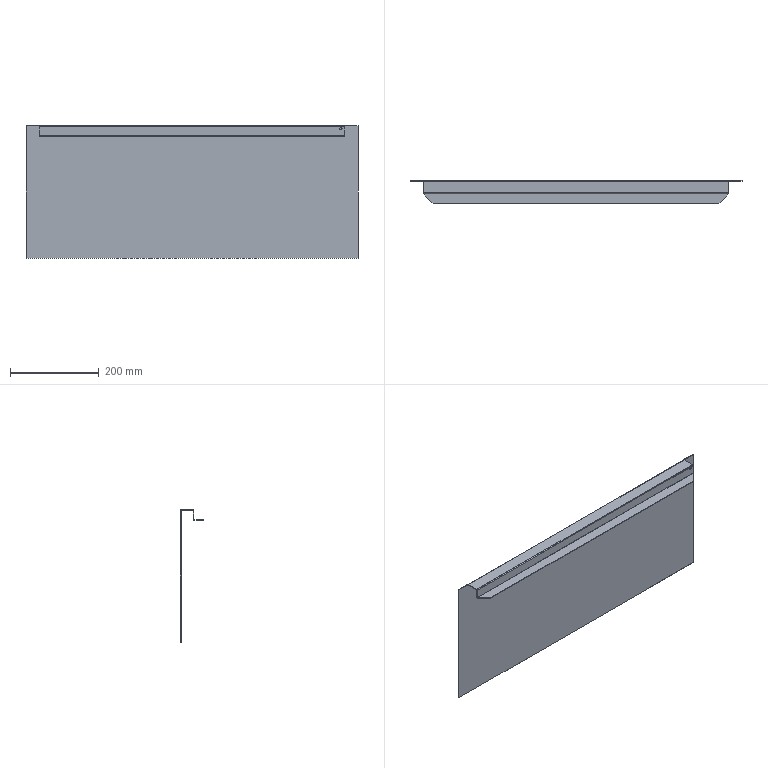Part | SolidWorks | features BaseBody 1, FlatPattern 1, FlattenBends 1, ProcessBends 1, SheetMetal 1 | 1 solid | 42 faces | box 750 x 52 x 298.5 mm | volume 408654 mm3 | plane 32 | cylinder 8 | spline 2 | commonest cylinder face diameters 0.6 x3 3.6 x3 5.2 x2
STEP:
#1=CARTESIAN_POINT('',(333.9,721.5,294.));
#2=VERTEX_POINT('',#1);
#3=CARTESIAN_POINT('',(339.1,721.5,294.));
#4=VERTEX_POINT('',#3);
#5=CARTESIAN_POINT('',(336.5,721.5,294.));
#6=DIRECTION('',(0.,-1.,0.));
#7=DIRECTION('',(0.,0.,1.));
#8=AXIS2_PLACEMENT_3D('',#5,#6,#7);
#9=CIRCLE('',#8,2.6);
#10=EDGE_CURVE('',#2,#4,#9,.T.);
#11=ORIENTED_EDGE('',*,*,#10,.F.);
#12=CARTESIAN_POINT('',(333.9,720.,294.));
#13=VERTEX_POINT('',#12);
#14=CARTESIAN_POINT('',(333.9,728.5,294.));
#15=DIRECTION('',(0.,-1.,0.));
#16=VECTOR('',#15,1000.);
#17=LINE('',#14,#16);
#18=EDGE_CURVE('',#2,#13,#17,.T.);
#19=ORIENTED_EDGE('',*,*,#18,.T.);
#20=CARTESIAN_POINT('',(339.1,720.,294.));
#21=VERTEX_POINT('',#20);
#22=CARTESIAN_POINT('',(336.5,720.,294.));
#23=DIRECTION('',(0.,-1.,0.));
#24=DIRECTION('',(0.,0.,1.));
#25=AXIS2_PLACEMENT_3D('',#22,#23,#24);
#26=CIRCLE('',#25,2.6);
#27=EDGE_CURVE('',#13,#21,#26,.T.);
#28=ORIENTED_EDGE('',*,*,#27,.T.);
#29=CARTESIAN_POINT('',(339.1,728.5,294.));
#30=DIRECTION('',(0.,-1.,0.));
#31=VECTOR('',#30,1000.);
#32=LINE('',#29,#31);
#33=EDGE_CURVE('',#4,#21,#32,.T.);
#34=ORIENTED_EDGE('',*,*,#33,.F.);
#35=EDGE_LOOP('',(#11,#19,#28,#34));
#36=FACE_OUTER_BOUND('',#35,.T.);
#37=CARTESIAN_POINT('',(336.5,728.5,294.));
#38=DIRECTION('',(0.,-1.,0.));
#39=DIRECTION('',(1.,0.,0.));
#40=AXIS2_PLACEMENT_3D('',#37,#38,#39);
#41=CYLINDRICAL_SURFACE('',#40,2.6);
#42=ADVANCED_FACE('',(#36),#41,.F.);
#43=CARTESIAN_POINT('',(323.,698.,276.5));
#44=VERTEX_POINT('',#43);
#45=CARTESIAN_POINT('',(-323.,698.,276.5));
#46=VERTEX_POINT('',#45);
#47=CARTESIAN_POINT('',(0.,698.,276.5));
#48=DIRECTION('',(-1.,0.,0.));
#49=VECTOR('',#48,1000.);
#50=LINE('',#47,#49);
#51=EDGE_CURVE('',#44,#46,#50,.T.);
#52=ORIENTED_EDGE('',*,*,#51,.F.);
#53=CARTESIAN_POINT('',(323.,698.,278.));
#54=VERTEX_POINT('',#53);
#55=CARTESIAN_POINT('',(323.,698.,1656.694));
#56=DIRECTION('',(0.,0.,-1.));
#57=VECTOR('',#56,1000.);
#58=LINE('',#55,#57);
#59=EDGE_CURVE('',#54,#44,#58,.T.);
#60=ORIENTED_EDGE('',*,*,#59,.F.);
#61=CARTESIAN_POINT('',(-323.,698.,278.));
#62=VERTEX_POINT('',#61);
#63=CARTESIAN_POINT('',(323.,698.,278.));
#64=DIRECTION('',(-1.,0.,0.));
#65=VECTOR('',#64,1000.);
#66=LINE('',#63,#65);
#67=EDGE_CURVE('',#54,#62,#66,.T.);
#68=ORIENTED_EDGE('',*,*,#67,.T.);
#69=CARTESIAN_POINT('',(-323.,698.,1656.694));
#70=DIRECTION('',(0.,0.,-1.));
#71=VECTOR('',#70,1000.);
#72=LINE('',#69,#71);
#73=EDGE_CURVE('',#62,#46,#72,.T.);
#74=ORIENTED_EDGE('',*,*,#73,.T.);
#75=EDGE_LOOP('',(#52,#60,#68,#74));
#76=FACE_OUTER_BOUND('',#75,.T.);
#77=CARTESIAN_POINT('',(323.,698.,1656.694));
#78=DIRECTION('',(0.,-1.,0.));
#79=DIRECTION('',(1.,0.,0.));
#80=AXIS2_PLACEMENT_3D('',#77,#78,#79);
#81=PLANE('',#80);
#82=ADVANCED_FACE('',(#76),#81,.T.);
#83=CARTESIAN_POINT('',(-344.503,719.7,276.5));
#84=VERTEX_POINT('',#83);
#85=CARTESIAN_POINT('',(186.011,184.32,276.5));
#86=DIRECTION('',(-0.7039,0.7103,0.));
#87=VECTOR('',#86,1000.);
#88=LINE('',#85,#87);
#89=EDGE_CURVE('',#46,#84,#88,.T.);
#90=ORIENTED_EDGE('',*,*,#89,.T.);
#91=CARTESIAN_POINT('',(344.503,719.7,276.5));
#92=VERTEX_POINT('',#91);
#93=CARTESIAN_POINT('',(-344.503,719.7,276.5));
#94=DIRECTION('',(1.,0.,0.));
#95=VECTOR('',#94,1000.);
#96=LINE('',#93,#95);
#97=EDGE_CURVE('',#84,#92,#96,.T.);
#98=ORIENTED_EDGE('',*,*,#97,.T.);
#99=CARTESIAN_POINT('',(-186.011,184.32,276.5));
#100=DIRECTION('',(0.7039,0.7103,0.));
#101=VECTOR('',#100,1000.);
#102=LINE('',#99,#101);
#103=EDGE_CURVE('',#44,#92,#102,.T.);
#104=ORIENTED_EDGE('',*,*,#103,.F.);
#105=ORIENTED_EDGE('',*,*,#51,.T.);
#106=EDGE_LOOP('',(#90,#98,#104,#105));
#107=FACE_OUTER_BOUND('',#106,.T.);
#108=CARTESIAN_POINT('',(0.,0.,276.5));
#109=DIRECTION('',(0.,0.,1.));
#110=DIRECTION('',(1.,0.,0.));
#111=AXIS2_PLACEMENT_3D('',#108,#109,#110);
#112=PLANE('',#111);
#113=ADVANCED_FACE('',(#107),#112,.F.);
#114=ORIENTED_EDGE('',*,*,#59,.T.);
#115=ORIENTED_EDGE('',*,*,#103,.T.);
#116=CARTESIAN_POINT('',(344.503,719.7,278.));
#117=VERTEX_POINT('',#116);
#118=CARTESIAN_POINT('',(344.503,719.7,278.));
#119=CARTESIAN_POINT('',(344.503,719.7,276.5));
#120=B_SPLINE_CURVE_WITH_KNOTS('',1,(#118,#119),.UNSPECIFIED.,.F.,.F.,(2,2),(0.,1.),.UNSPECIFIED.);
#121=EDGE_CURVE('',#117,#92,#120,.T.);
#122=ORIENTED_EDGE('',*,*,#121,.F.);
#123=CARTESIAN_POINT('',(-186.011,184.32,278.));
#124=DIRECTION('',(0.7039,0.7103,0.));
#125=VECTOR('',#124,1000.);
#126=LINE('',#123,#125);
#127=EDGE_CURVE('',#54,#117,#126,.T.);
#128=ORIENTED_EDGE('',*,*,#127,.F.);
#129=EDGE_LOOP('',(#114,#115,#122,#128));
#130=FACE_OUTER_BOUND('',#129,.T.);
#131=CARTESIAN_POINT('',(-186.011,184.32,1656.694));
#132=DIRECTION('',(-0.7103,0.7039,0.));
#133=DIRECTION('',(-0.7039,-0.7103,0.));
#134=AXIS2_PLACEMENT_3D('',#131,#132,#133);
#135=PLANE('',#134);
#136=ADVANCED_FACE('',(#130),#135,.F.);
#137=CARTESIAN_POINT('',(-344.503,719.7,278.));
#138=VERTEX_POINT('',#137);
#139=CARTESIAN_POINT('',(-344.503,719.7,278.));
#140=DIRECTION('',(1.,0.,0.));
#141=VECTOR('',#140,1000.);
#142=LINE('',#139,#141);
#143=EDGE_CURVE('',#138,#117,#142,.T.);
#144=ORIENTED_EDGE('',*,*,#143,.F.);
#145=CARTESIAN_POINT('',(186.011,184.32,278.));
#146=DIRECTION('',(-0.7039,0.7103,0.));
#147=VECTOR('',#146,1000.);
#148=LINE('',#145,#147);
#149=EDGE_CURVE('',#62,#138,#148,.T.);
#150=ORIENTED_EDGE('',*,*,#149,.F.);
#151=ORIENTED_EDGE('',*,*,#67,.F.);
#152=ORIENTED_EDGE('',*,*,#127,.T.);
#153=EDGE_LOOP('',(#144,#150,#151,#152));
#154=FACE_OUTER_BOUND('',#153,.T.);
#155=CARTESIAN_POINT('',(0.,0.,278.));
#156=DIRECTION('',(0.,0.,1.));
#157=DIRECTION('',(1.,0.,0.));
#158=AXIS2_PLACEMENT_3D('',#155,#156,#157);
#159=PLANE('',#158);
#160=ADVANCED_FACE('',(#154),#159,.T.);
#161=ORIENTED_EDGE('',*,*,#89,.F.);
#162=ORIENTED_EDGE('',*,*,#73,.F.);
#163=ORIENTED_EDGE('',*,*,#149,.T.);
#164=CARTESIAN_POINT('',(-344.503,719.7,278.));
#165=CARTESIAN_POINT('',(-344.503,719.7,277.5));
#166=CARTESIAN_POINT('',(-344.503,719.7,277.));
#167=CARTESIAN_POINT('',(-344.503,719.7,276.5));
#168=B_SPLINE_CURVE_WITH_KNOTS('',3,(#164,#165,#166,#167),.UNSPECIFIED.,.F.,.F.,(4,4),(0.,1.),.UNSPECIFIED.);
#169=EDGE_CURVE('',#138,#84,#168,.T.);
#170=ORIENTED_EDGE('',*,*,#169,.T.);
#171=EDGE_LOOP('',(#161,#162,#163,#170));
#172=FACE_OUTER_BOUND('',#171,.T.);
#173=CARTESIAN_POINT('',(186.011,184.32,1656.694));
#174=DIRECTION('',(-0.7103,-0.7039,0.));
#175=DIRECTION('',(0.7039,-0.7103,0.));
#176=AXIS2_PLACEMENT_3D('',#173,#174,#175);
#177=PLANE('',#176);
#178=ADVANCED_FACE('',(#172),#177,.T.);
#179=ORIENTED_EDGE('',*,*,#18,.F.);
#180=CARTESIAN_POINT('',(336.5,721.5,294.));
#181=DIRECTION('',(0.,-1.,0.));
#182=DIRECTION('',(0.,0.,1.));
#183=AXIS2_PLACEMENT_3D('',#180,#181,#182);
#184=CIRCLE('',#183,2.6);
#185=EDGE_CURVE('',#4,#2,#184,.T.);
#186=ORIENTED_EDGE('',*,*,#185,.F.);
#187=ORIENTED_EDGE('',*,*,#33,.T.);
#188=CARTESIAN_POINT('',(336.5,720.,294.));
#189=DIRECTION('',(0.,-1.,0.));
#190=DIRECTION('',(0.,0.,1.));
#191=AXIS2_PLACEMENT_3D('',#188,#189,#190);
#192=CIRCLE('',#191,2.6);
#193=EDGE_CURVE('',#21,#13,#192,.T.);
#194=ORIENTED_EDGE('',*,*,#193,.T.);
#195=EDGE_LOOP('',(#179,#186,#187,#194));
#196=FACE_OUTER_BOUND('',#195,.T.);
#197=CARTESIAN_POINT('',(336.5,728.5,294.));
#198=DIRECTION('',(0.,-1.,0.));
#199=DIRECTION('',(1.,0.,0.));
#200=AXIS2_PLACEMENT_3D('',#197,#198,#199);
#201=CYLINDRICAL_SURFACE('',#200,2.6);
#202=ADVANCED_FACE('',(#196),#201,.F.);
#203=CARTESIAN_POINT('',(344.8,721.5,298.2));
#204=VERTEX_POINT('',#203);
#205=CARTESIAN_POINT('',(344.8,720.,298.2));
#206=VERTEX_POINT('',#205);
#207=CARTESIAN_POINT('',(344.8,2099.774,298.2));
#208=DIRECTION('',(0.,-1.,0.));
#209=VECTOR('',#208,1000.);
#210=LINE('',#207,#209);
#211=EDGE_CURVE('',#204,#206,#210,.T.);
#212=ORIENTED_EDGE('',*,*,#211,.T.);
#213=CARTESIAN_POINT('',(344.8,720.,278.3));
#214=VERTEX_POINT('',#213);
#215=CARTESIAN_POINT('',(344.8,720.,278.));
#216=DIRECTION('',(0.,0.,-1.));
#217=VECTOR('',#216,1000.);
#218=LINE('',#215,#217);
#219=EDGE_CURVE('',#206,#214,#218,.T.);
#220=ORIENTED_EDGE('',*,*,#219,.T.);
#221=CARTESIAN_POINT('',(344.8,721.5,278.3));
#222=VERTEX_POINT('',#221);
#223=CARTESIAN_POINT('',(344.8,2099.774,278.3));
#224=DIRECTION('',(0.,-1.,0.));
#225=VECTOR('',#224,1000.);
#226=LINE('',#223,#225);
#227=EDGE_CURVE('',#222,#214,#226,.T.);
#228=ORIENTED_EDGE('',*,*,#227,.F.);
#229=CARTESIAN_POINT('',(344.8,721.5,278.));
#230=DIRECTION('',(0.,0.,-1.));
#231=VECTOR('',#230,1000.);
#232=LINE('',#229,#231);
#233=EDGE_CURVE('',#204,#222,#232,.T.);
#234=ORIENTED_EDGE('',*,*,#233,.F.);
#235=EDGE_LOOP('',(#212,#220,#228,#234));
#236=FACE_OUTER_BOUND('',#235,.T.);
#237=CARTESIAN_POINT('',(344.8,2099.774,278.));
#238=DIRECTION('',(-1.,0.,0.));
#239=DIRECTION('',(0.,0.,-1.));
#240=AXIS2_PLACEMENT_3D('',#237,#238,#239);
#241=PLANE('',#240);
#242=ADVANCED_FACE('',(#236),#241,.F.);
#243=ORIENTED_EDGE('',*,*,#193,.F.);
#244=ORIENTED_EDGE('',*,*,#27,.F.);
#245=EDGE_LOOP('',(#243,#244));
#246=FACE_BOUND('',#245,.T.);
#247=CARTESIAN_POINT('',(-344.8,720.,298.2));
#248=VERTEX_POINT('',#247);
#249=CARTESIAN_POINT('',(-344.8,720.,278.3));
#250=VERTEX_POINT('',#249);
#251=CARTESIAN_POINT('',(-344.8,720.,300.));
#252=DIRECTION('',(0.,0.,-1.));
#253=VECTOR('',#252,1000.);
#254=LINE('',#251,#253);
#255=EDGE_CURVE('',#248,#250,#254,.T.);
#256=ORIENTED_EDGE('',*,*,#255,.T.);
#257=CARTESIAN_POINT('',(-344.8,720.,278.3));
#258=DIRECTION('',(1.,0.,0.));
#259=VECTOR('',#258,1000.);
#260=LINE('',#257,#259);
#261=EDGE_CURVE('',#250,#214,#260,.T.);
#262=ORIENTED_EDGE('',*,*,#261,.T.);
#263=ORIENTED_EDGE('',*,*,#219,.F.);
#264=CARTESIAN_POINT('',(344.8,720.,298.2));
#265=DIRECTION('',(-1.,0.,0.));
#266=VECTOR('',#265,1000.);
#267=LINE('',#264,#266);
#268=EDGE_CURVE('',#206,#248,#267,.T.);
#269=ORIENTED_EDGE('',*,*,#268,.T.);
#270=EDGE_LOOP('',(#256,#262,#263,#269));
#271=FACE_OUTER_BOUND('',#270,.T.);
#272=CARTESIAN_POINT('',(345.,720.,278.));
#273=DIRECTION('',(0.,1.,0.));
#274=DIRECTION('',(0.,0.,1.));
#275=AXIS2_PLACEMENT_3D('',#272,#273,#274);
#276=PLANE('',#275);
#277=ADVANCED_FACE('',(#246,#271),#276,.F.);
#278=CARTESIAN_POINT('',(-344.8,721.5,278.3));
#279=VERTEX_POINT('',#278);
#280=CARTESIAN_POINT('',(-344.8,2099.774,278.3));
#281=DIRECTION('',(0.,-1.,0.));
#282=VECTOR('',#281,1000.);
#283=LINE('',#280,#282);
#284=EDGE_CURVE('',#279,#250,#283,.T.);
#285=ORIENTED_EDGE('',*,*,#284,.T.);
#286=ORIENTED_EDGE('',*,*,#255,.F.);
#287=CARTESIAN_POINT('',(-344.8,721.5,298.2));
#288=VERTEX_POINT('',#287);
#289=CARTESIAN_POINT('',(-344.8,2099.774,298.2));
#290=DIRECTION('',(0.,-1.,0.));
#291=VECTOR('',#290,1000.);
#292=LINE('',#289,#291);
#293=EDGE_CURVE('',#288,#248,#292,.T.);
#294=ORIENTED_EDGE('',*,*,#293,.F.);
#295=CARTESIAN_POINT('',(-344.8,721.5,278.));
#296=DIRECTION('',(0.,0.,1.));
#297=VECTOR('',#296,1000.);
#298=LINE('',#295,#297);
#299=EDGE_CURVE('',#279,#288,#298,.T.);
#300=ORIENTED_EDGE('',*,*,#299,.F.);
#301=EDGE_LOOP('',(#285,#286,#294,#300));
#302=FACE_OUTER_BOUND('',#301,.T.);
#303=CARTESIAN_POINT('',(-344.8,2099.774,278.));
#304=DIRECTION('',(1.,0.,0.));
#305=DIRECTION('',(0.,0.,1.));
#306=AXIS2_PLACEMENT_3D('',#303,#304,#305);
#307=PLANE('',#306);
#308=ADVANCED_FACE('',(#302),#307,.F.);
#309=CARTESIAN_POINT('',(-344.8,721.5,278.3));
#310=DIRECTION('',(1.,0.,0.));
#311=VECTOR('',#310,1000.);
#312=LINE('',#309,#311);
#313=EDGE_CURVE('',#279,#222,#312,.T.);
#314=ORIENTED_EDGE('',*,*,#313,.F.);
#315=ORIENTED_EDGE('',*,*,#299,.T.);
#316=CARTESIAN_POINT('',(344.8,721.5,298.2));
#317=DIRECTION('',(-1.,0.,0.));
#318=VECTOR('',#317,1000.);
#319=LINE('',#316,#318);
#320=EDGE_CURVE('',#204,#288,#319,.T.);
#321=ORIENTED_EDGE('',*,*,#320,.F.);
#322=ORIENTED_EDGE('',*,*,#233,.T.);
#323=EDGE_LOOP('',(#314,#315,#321,#322));
#324=FACE_OUTER_BOUND('',#323,.T.);
#325=ORIENTED_EDGE('',*,*,#185,.T.);
#326=ORIENTED_EDGE('',*,*,#10,.T.);
#327=EDGE_LOOP('',(#325,#326));
#328=FACE_BOUND('',#327,.T.);
#329=CARTESIAN_POINT('',(345.,721.5,278.));
#330=DIRECTION('',(0.,1.,0.));
#331=DIRECTION('',(0.,0.,1.));
#332=AXIS2_PLACEMENT_3D('',#329,#330,#331);
#333=PLANE('',#332);
#334=ADVANCED_FACE('',(#324,#328),#333,.T.);
#335=CARTESIAN_POINT('',(344.8,748.2,298.5));
#336=VERTEX_POINT('',#335);
#337=CARTESIAN_POINT('',(344.8,721.8,298.5));
#338=VERTEX_POINT('',#337);
#339=CARTESIAN_POINT('',(344.8,0.,298.5));
#340=DIRECTION('',(0.,-1.,0.));
#341=VECTOR('',#340,1000.);
#342=LINE('',#339,#341);
#343=EDGE_CURVE('',#336,#338,#342,.T.);
#344=ORIENTED_EDGE('',*,*,#343,.T.);
#345=CARTESIAN_POINT('',(-344.8,721.8,298.5));
#346=VERTEX_POINT('',#345);
#347=CARTESIAN_POINT('',(344.8,721.8,298.5));
#348=DIRECTION('',(-1.,0.,0.));
#349=VECTOR('',#348,1000.);
#350=LINE('',#347,#349);
#351=EDGE_CURVE('',#338,#346,#350,.T.);
#352=ORIENTED_EDGE('',*,*,#351,.T.);
#353=CARTESIAN_POINT('',(-344.8,748.2,298.5));
#354=VERTEX_POINT('',#353);
#355=CARTESIAN_POINT('',(-344.8,0.,298.5));
#356=DIRECTION('',(0.,1.,0.));
#357=VECTOR('',#356,1000.);
#358=LINE('',#355,#357);
#359=EDGE_CURVE('',#346,#354,#358,.T.);
#360=ORIENTED_EDGE('',*,*,#359,.T.);
#361=CARTESIAN_POINT('',(344.8,748.2,298.5));
#362=DIRECTION('',(-1.,0.,0.));
#363=VECTOR('',#362,1000.);
#364=LINE('',#361,#363);
#365=EDGE_CURVE('',#336,#354,#364,.T.);
#366=ORIENTED_EDGE('',*,*,#365,.F.);
#367=EDGE_LOOP('',(#344,#352,#360,#366));
#368=FACE_OUTER_BOUND('',#367,.T.);
#369=CARTESIAN_POINT('',(0.,0.,298.5));
#370=DIRECTION('',(0.,0.,-1.));
#371=DIRECTION('',(-1.,0.,0.));
#372=AXIS2_PLACEMENT_3D('',#369,#370,#371);
#373=PLANE('',#372);
#374=ADVANCED_FACE('',(#368),#373,.T.);
#375=CARTESIAN_POINT('',(344.8,748.2,300.));
#376=VERTEX_POINT('',#375);
#377=CARTESIAN_POINT('',(344.8,748.2,-1080.21));
#378=DIRECTION('',(0.,0.,1.));
#379=VECTOR('',#378,1000.);
#380=LINE('',#377,#379);
#381=EDGE_CURVE('',#336,#376,#380,.T.);
#382=ORIENTED_EDGE('',*,*,#381,.T.);
#383=CARTESIAN_POINT('',(344.8,721.8,300.));
#384=VERTEX_POINT('',#383);
#385=CARTESIAN_POINT('',(344.8,748.5,300.));
#386=DIRECTION('',(0.,-1.,0.));
#387=VECTOR('',#386,1000.);
#388=LINE('',#385,#387);
#389=EDGE_CURVE('',#376,#384,#388,.T.);
#390=ORIENTED_EDGE('',*,*,#389,.T.);
#391=CARTESIAN_POINT('',(344.8,721.8,-1080.21));
#392=DIRECTION('',(0.,0.,1.));
#393=VECTOR('',#392,1000.);
#394=LINE('',#391,#393);
#395=EDGE_CURVE('',#338,#384,#394,.T.);
#396=ORIENTED_EDGE('',*,*,#395,.F.);
#397=ORIENTED_EDGE('',*,*,#343,.F.);
#398=EDGE_LOOP('',(#382,#390,#396,#397));
#399=FACE_OUTER_BOUND('',#398,.T.);
#400=CARTESIAN_POINT('',(344.8,0.,-1080.21));
#401=DIRECTION('',(-1.,0.,0.));
#402=DIRECTION('',(0.,-1.,0.));
#403=AXIS2_PLACEMENT_3D('',#400,#401,#402);
#404=PLANE('',#403);
#405=ADVANCED_FACE('',(#399),#404,.F.);
#406=CARTESIAN_POINT('',(-344.8,721.8,300.));
#407=VERTEX_POINT('',#406);
#408=CARTESIAN_POINT('',(-344.8,721.8,-1080.21));
#409=DIRECTION('',(0.,0.,1.));
#410=VECTOR('',#409,1000.);
#411=LINE('',#408,#410);
#412=EDGE_CURVE('',#346,#407,#411,.T.);
#413=ORIENTED_EDGE('',*,*,#412,.T.);
#414=CARTESIAN_POINT('',(-344.8,748.2,300.));
#415=VERTEX_POINT('',#414);
#416=CARTESIAN_POINT('',(-344.8,748.5,300.));
#417=DIRECTION('',(0.,1.,0.));
#418=VECTOR('',#417,1000.);
#419=LINE('',#416,#418);
#420=EDGE_CURVE('',#407,#415,#419,.T.);
#421=ORIENTED_EDGE('',*,*,#420,.T.);
#422=CARTESIAN_POINT('',(-344.8,748.2,-1080.21));
#423=DIRECTION('',(0.,0.,1.));
#424=VECTOR('',#423,1000.);
#425=LINE('',#422,#424);
#426=EDGE_CURVE('',#354,#415,#425,.T.);
#427=ORIENTED_EDGE('',*,*,#426,.F.);
#428=ORIENTED_EDGE('',*,*,#359,.F.);
#429=EDGE_LOOP('',(#413,#421,#427,#428));
#430=FACE_OUTER_BOUND('',#429,.T.);
#431=CARTESIAN_POINT('',(-344.8,0.,-1080.21));
#432=DIRECTION('',(1.,0.,0.));
#433=DIRECTION('',(0.,1.,0.));
#434=AXIS2_PLACEMENT_3D('',#431,#432,#433);
#435=PLANE('',#434);
#436=ADVANCED_FACE('',(#430),#435,.F.);
#437=CARTESIAN_POINT('',(344.8,721.8,300.));
#438=DIRECTION('',(-1.,0.,0.));
#439=VECTOR('',#438,1000.);
#440=LINE('',#437,#439);
#441=EDGE_CURVE('',#384,#407,#440,.T.);
#442=ORIENTED_EDGE('',*,*,#441,.F.);
#443=ORIENTED_EDGE('',*,*,#389,.F.);
#444=CARTESIAN_POINT('',(344.8,748.2,300.));
#445=DIRECTION('',(-1.,0.,0.));
#446=VECTOR('',#445,1000.);
#447=LINE('',#444,#446);
#448=EDGE_CURVE('',#376,#415,#447,.T.);
#449=ORIENTED_EDGE('',*,*,#448,.T.);
#450=ORIENTED_EDGE('',*,*,#420,.F.);
#451=EDGE_LOOP('',(#442,#443,#449,#450));
#452=FACE_OUTER_BOUND('',#451,.T.);
#453=CARTESIAN_POINT('',(0.,0.,300.));
#454=DIRECTION('',(0.,0.,-1.));
#455=DIRECTION('',(-1.,0.,0.));
#456=AXIS2_PLACEMENT_3D('',#453,#454,#455);
#457=PLANE('',#456);
#458=ADVANCED_FACE('',(#452),#457,.F.);
#459=CARTESIAN_POINT('',(345.2,750.,298.));
#460=VERTEX_POINT('',#459);
#461=CARTESIAN_POINT('',(345.2,750.,300.));
#462=VERTEX_POINT('',#461);
#463=CARTESIAN_POINT('',(345.2,750.,300.));
#464=DIRECTION('',(0.,0.,1.));
#465=VECTOR('',#464,1000.);
#466=LINE('',#463,#465);
#467=EDGE_CURVE('',#460,#462,#466,.T.);
#468=ORIENTED_EDGE('',*,*,#467,.F.);
#469=CARTESIAN_POINT('',(345.2,748.5,298.));
#470=VERTEX_POINT('',#469);
#471=CARTESIAN_POINT('',(345.2,-864.438,298.));
#472=DIRECTION('',(0.,1.,0.));
#473=VECTOR('',#472,1000.);
#474=LINE('',#471,#473);
#475=EDGE_CURVE('',#470,#460,#474,.T.);
#476=ORIENTED_EDGE('',*,*,#475,.F.);
#477=CARTESIAN_POINT('',(345.2,748.5,300.));
#478=VERTEX_POINT('',#477);
#479=CARTESIAN_POINT('',(345.2,748.5,300.5));
#480=DIRECTION('',(0.,0.,1.));
#481=VECTOR('',#480,1000.);
#482=LINE('',#479,#481);
#483=EDGE_CURVE('',#470,#478,#482,.T.);
#484=ORIENTED_EDGE('',*,*,#483,.T.);
#485=CARTESIAN_POINT('',(345.2,-864.438,300.));
#486=DIRECTION('',(0.,1.,0.));
#487=VECTOR('',#486,1000.);
#488=LINE('',#485,#487);
#489=EDGE_CURVE('',#478,#462,#488,.T.);
#490=ORIENTED_EDGE('',*,*,#489,.T.);
#491=EDGE_LOOP('',(#468,#476,#484,#490));
#492=FACE_OUTER_BOUND('',#491,.T.);
#493=CARTESIAN_POINT('',(345.2,-864.438,300.5));
#494=DIRECTION('',(-1.,0.,0.));
#495=DIRECTION('',(0.,0.,1.));
#496=AXIS2_PLACEMENT_3D('',#493,#494,#495);
#497=PLANE('',#496);
#498=ADVANCED_FACE('',(#492),#497,.T.);
#499=CARTESIAN_POINT('',(375.,748.5,300.));
#500=VERTEX_POINT('',#499);
#501=CARTESIAN_POINT('',(375.,750.,300.));
#502=VERTEX_POINT('',#501);
#503=CARTESIAN_POINT('',(375.,-864.438,300.));
#504=DIRECTION('',(0.,1.,0.));
#505=VECTOR('',#504,1000.);
#506=LINE('',#503,#505);
#507=EDGE_CURVE('',#500,#502,#506,.T.);
#508=ORIENTED_EDGE('',*,*,#507,.T.);
#509=CARTESIAN_POINT('',(-375.,750.,300.));
#510=DIRECTION('',(-1.,0.,0.));
#511=VECTOR('',#510,1000.);
#512=LINE('',#509,#511);
#513=EDGE_CURVE('',#502,#462,#512,.T.);
#514=ORIENTED_EDGE('',*,*,#513,.T.);
#515=ORIENTED_EDGE('',*,*,#489,.F.);
#516=CARTESIAN_POINT('',(435.,748.5,300.));
#517=DIRECTION('',(-1.,0.,0.));
#518=VECTOR('',#517,1000.);
#519=LINE('',#516,#518);
#520=EDGE_CURVE('',#500,#478,#519,.T.);
#521=ORIENTED_EDGE('',*,*,#520,.F.);
#522=EDGE_LOOP('',(#508,#514,#515,#521));
#523=FACE_OUTER_BOUND('',#522,.T.);
#524=CARTESIAN_POINT('',(435.,-864.438,300.));
#525=DIRECTION('',(0.,0.,-1.));
#526=DIRECTION('',(-1.,0.,0.));
#527=AXIS2_PLACEMENT_3D('',#524,#525,#526);
#528=PLANE('',#527);
#529=ADVANCED_FACE('',(#523),#528,.F.);
#530=CARTESIAN_POINT('',(375.,748.5,1.5));
#531=VERTEX_POINT('',#530);
#532=CARTESIAN_POINT('',(375.,750.,1.5));
#533=VERTEX_POINT('',#532);
#534=CARTESIAN_POINT('',(375.,-864.438,1.5));
#535=DIRECTION('',(0.,1.,0.));
#536=VECTOR('',#535,1000.);
#537=LINE('',#534,#536);
#538=EDGE_CURVE('',#531,#533,#537,.T.);
#539=ORIENTED_EDGE('',*,*,#538,.T.);
#540=CARTESIAN_POINT('',(375.,750.,300.));
#541=DIRECTION('',(0.,0.,-1.));
#542=VECTOR('',#541,1000.);
#543=LINE('',#540,#542);
#544=EDGE_CURVE('',#502,#533,#543,.T.);
#545=ORIENTED_EDGE('',*,*,#544,.F.);
#546=ORIENTED_EDGE('',*,*,#507,.F.);
#547=CARTESIAN_POINT('',(375.,748.5,300.));
#548=DIRECTION('',(0.,0.,1.));
#549=VECTOR('',#548,1000.);
#550=LINE('',#547,#549);
#551=EDGE_CURVE('',#531,#500,#550,.T.);
#552=ORIENTED_EDGE('',*,*,#551,.F.);
#553=EDGE_LOOP('',(#539,#545,#546,#552));
#554=FACE_OUTER_BOUND('',#553,.T.);
#555=CARTESIAN_POINT('',(375.,-864.438,300.));
#556=DIRECTION('',(-1.,0.,0.));
#557=DIRECTION('',(0.,0.,1.));
#558=AXIS2_PLACEMENT_3D('',#555,#556,#557);
#559=PLANE('',#558);
#560=ADVANCED_FACE('',(#554),#559,.F.);
#561=CARTESIAN_POINT('',(-375.,750.,1.5));
#562=VERTEX_POINT('',#561);
#563=CARTESIAN_POINT('',(-375.,750.,1.5));
#564=DIRECTION('',(-1.,0.,0.));
#565=VECTOR('',#564,1000.);
#566=LINE('',#563,#565);
#567=EDGE_CURVE('',#533,#562,#566,.T.);
#568=ORIENTED_EDGE('',*,*,#567,.F.);
#569=ORIENTED_EDGE('',*,*,#538,.F.);
#570=CARTESIAN_POINT('',(-375.,748.5,1.5));
#571=VERTEX_POINT('',#570);
#572=CARTESIAN_POINT('',(0.,748.5,1.5));
#573=DIRECTION('',(-1.,0.,0.));
#574=VECTOR('',#573,1000.);
#575=LINE('',#572,#574);
#576=EDGE_CURVE('',#531,#571,#575,.T.);
#577=ORIENTED_EDGE('',*,*,#576,.T.);
#578=CARTESIAN_POINT('',(-375.,-864.438,1.5));
#579=DIRECTION('',(0.,1.,0.));
#580=VECTOR('',#579,1000.);
#581=LINE('',#578,#580);
#582=EDGE_CURVE('',#571,#562,#581,.T.);
#583=ORIENTED_EDGE('',*,*,#582,.T.);
#584=EDGE_LOOP('',(#568,#569,#577,#583));
#585=FACE_OUTER_BOUND('',#584,.T.);
#586=CARTESIAN_POINT('',(0.,-864.438,1.5));
#587=DIRECTION('',(0.,0.,-1.));
#588=DIRECTION('',(-1.,0.,0.));
#589=AXIS2_PLACEMENT_3D('',#586,#587,#588);
#590=PLANE('',#589);
#591=ADVANCED_FACE('',(#585),#590,.T.);
#592=CARTESIAN_POINT('',(-375.,748.5,300.));
#593=VERTEX_POINT('',#592);
#594=CARTESIAN_POINT('',(-375.,750.,300.));
#595=VERTEX_POINT('',#594);
#596=CARTESIAN_POINT('',(-375.,-864.438,300.));
#597=DIRECTION('',(0.,1.,0.));
#598=VECTOR('',#597,1000.);
#599=LINE('',#596,#598);
#600=EDGE_CURVE('',#593,#595,#599,.T.);
#601=ORIENTED_EDGE('',*,*,#600,.T.);
#602=CARTESIAN_POINT('',(-375.,750.,300.));
#603=DIRECTION('',(0.,0.,-1.));
#604=VECTOR('',#603,1000.);
#605=LINE('',#602,#604);
#606=EDGE_CURVE('',#595,#562,#605,.T.);
#607=ORIENTED_EDGE('',*,*,#606,.T.);
#608=ORIENTED_EDGE('',*,*,#582,.F.);
#609=CARTESIAN_POINT('',(-375.,748.5,300.));
#610=DIRECTION('',(0.,0.,-1.));
#611=VECTOR('',#610,1000.);
#612=LINE('',#609,#611);
#613=EDGE_CURVE('',#593,#571,#612,.T.);
#614=ORIENTED_EDGE('',*,*,#613,.F.);
#615=EDGE_LOOP('',(#601,#607,#608,#614));
#616=FACE_OUTER_BOUND('',#615,.T.);
#617=CARTESIAN_POINT('',(-375.,-864.438,300.));
#618=DIRECTION('',(1.,0.,0.));
#619=DIRECTION('',(0.,0.,-1.));
#620=AXIS2_PLACEMENT_3D('',#617,#618,#619);
#621=PLANE('',#620);
#622=ADVANCED_FACE('',(#616),#621,.F.);
#623=CARTESIAN_POINT('',(-345.2,748.5,300.));
#624=VERTEX_POINT('',#623);
#625=CARTESIAN_POINT('',(-345.2,750.,300.));
#626=VERTEX_POINT('',#625);
#627=CARTESIAN_POINT('',(-345.2,-864.438,300.));
#628=DIRECTION('',(0.,1.,0.));
#629=VECTOR('',#628,1000.);
#630=LINE('',#627,#629);
#631=EDGE_CURVE('',#624,#626,#630,.T.);
#632=ORIENTED_EDGE('',*,*,#631,.T.);
#633=CARTESIAN_POINT('',(-375.,750.,300.));
#634=DIRECTION('',(-1.,0.,0.));
#635=VECTOR('',#634,1000.);
#636=LINE('',#633,#635);
#637=EDGE_CURVE('',#626,#595,#636,.T.);
#638=ORIENTED_EDGE('',*,*,#637,.T.);
#639=ORIENTED_EDGE('',*,*,#600,.F.);
#640=CARTESIAN_POINT('',(-435.,748.5,300.));
#641=DIRECTION('',(-1.,0.,0.));
#642=VECTOR('',#641,1000.);
#643=LINE('',#640,#642);
#644=EDGE_CURVE('',#624,#593,#643,.T.);
#645=ORIENTED_EDGE('',*,*,#644,.F.);
#646=EDGE_LOOP('',(#632,#638,#639,#645));
#647=FACE_OUTER_BOUND('',#646,.T.);
#648=CARTESIAN_POINT('',(-435.,-864.438,300.));
#649=DIRECTION('',(0.,0.,-1.));
#650=DIRECTION('',(-1.,0.,0.));
#651=AXIS2_PLACEMENT_3D('',#648,#649,#650);
#652=PLANE('',#651);
#653=ADVANCED_FACE('',(#647),#652,.F.);
#654=CARTESIAN_POINT('',(-345.2,750.,298.));
#655=VERTEX_POINT('',#654);
#656=CARTESIAN_POINT('',(-345.2,750.,300.));
#657=DIRECTION('',(0.,0.,-1.));
#658=VECTOR('',#657,1000.);
#659=LINE('',#656,#658);
#660=EDGE_CURVE('',#626,#655,#659,.T.);
#661=ORIENTED_EDGE('',*,*,#660,.F.);
#662=ORIENTED_EDGE('',*,*,#631,.F.);
#663=CARTESIAN_POINT('',(-345.2,748.5,298.));
#664=VERTEX_POINT('',#663);
#665=CARTESIAN_POINT('',(-345.2,748.5,300.5));
#666=DIRECTION('',(0.,0.,-1.));
#667=VECTOR('',#666,1000.);
#668=LINE('',#665,#667);
#669=EDGE_CURVE('',#624,#664,#668,.T.);
#670=ORIENTED_EDGE('',*,*,#669,.T.);
#671=CARTESIAN_POINT('',(-345.2,-864.438,298.));
#672=DIRECTION('',(0.,1.,0.));
#673=VECTOR('',#672,1000.);
#674=LINE('',#671,#673);
#675=EDGE_CURVE('',#664,#655,#674,.T.);
#676=ORIENTED_EDGE('',*,*,#675,.T.);
#677=EDGE_LOOP('',(#661,#662,#670,#676));
#678=FACE_OUTER_BOUND('',#677,.T.);
#679=CARTESIAN_POINT('',(-345.2,-864.438,300.5));
#680=DIRECTION('',(1.,0.,0.));
#681=DIRECTION('',(0.,0.,-1.));
#682=AXIS2_PLACEMENT_3D('',#679,#680,#681);
#683=PLANE('',#682);
#684=ADVANCED_FACE('',(#678),#683,.T.);
#685=CARTESIAN_POINT('',(-344.8,750.,298.));
#686=VERTEX_POINT('',#685);
#687=CARTESIAN_POINT('',(-375.,750.,298.));
#688=DIRECTION('',(1.,0.,0.));
#689=VECTOR('',#688,1000.);
#690=LINE('',#687,#689);
#691=EDGE_CURVE('',#655,#686,#690,.T.);
#692=ORIENTED_EDGE('',*,*,#691,.F.);
#693=ORIENTED_EDGE('',*,*,#675,.F.);
#694=CARTESIAN_POINT('',(-344.8,748.5,298.));
#695=VERTEX_POINT('',#694);
#696=CARTESIAN_POINT('',(-344.8,748.5,298.));
#697=DIRECTION('',(1.,0.,0.));
#698=VECTOR('',#697,1000.);
#699=LINE('',#696,#698);
#700=EDGE_CURVE('',#664,#695,#699,.T.);
#701=ORIENTED_EDGE('',*,*,#700,.T.);
#702=CARTESIAN_POINT('',(-344.8,-864.438,298.));
#703=DIRECTION('',(0.,1.,0.));
#704=VECTOR('',#703,1000.);
#705=LINE('',#702,#704);
#706=EDGE_CURVE('',#695,#686,#705,.T.);
#707=ORIENTED_EDGE('',*,*,#706,.T.);
#708=EDGE_LOOP('',(#692,#693,#701,#707));
#709=FACE_OUTER_BOUND('',#708,.T.);
#710=CARTESIAN_POINT('',(-344.8,-864.438,298.));
#711=DIRECTION('',(0.,0.,1.));
#712=DIRECTION('',(1.,0.,0.));
#713=AXIS2_PLACEMENT_3D('',#710,#711,#712);
#714=PLANE('',#713);
#715=ADVANCED_FACE('',(#709),#714,.T.);
#716=CARTESIAN_POINT('',(344.8,750.,298.));
#717=VERTEX_POINT('',#716);
#718=CARTESIAN_POINT('',(-375.,750.,298.));
#719=DIRECTION('',(1.,0.,0.));
#720=VECTOR('',#719,1000.);
#721=LINE('',#718,#720);
#722=EDGE_CURVE('',#717,#460,#721,.T.);
#723=ORIENTED_EDGE('',*,*,#722,.F.);
#724=CARTESIAN_POINT('',(344.8,748.5,298.));
#725=VERTEX_POINT('',#724);
#726=CARTESIAN_POINT('',(344.8,-864.438,298.));
#727=DIRECTION('',(0.,1.,0.));
#728=VECTOR('',#727,1000.);
#729=LINE('',#726,#728);
#730=EDGE_CURVE('',#725,#717,#729,.T.);
#731=ORIENTED_EDGE('',*,*,#730,.F.);
#732=CARTESIAN_POINT('',(344.8,748.5,298.));
#733=DIRECTION('',(1.,0.,0.));
#734=VECTOR('',#733,1000.);
#735=LINE('',#732,#734);
#736=EDGE_CURVE('',#725,#470,#735,.T.);
#737=ORIENTED_EDGE('',*,*,#736,.T.);
#738=ORIENTED_EDGE('',*,*,#475,.T.);
#739=EDGE_LOOP('',(#723,#731,#737,#738));
#740=FACE_OUTER_BOUND('',#739,.T.);
#741=CARTESIAN_POINT('',(344.8,-864.438,298.));
#742=DIRECTION('',(0.,0.,1.));
#743=DIRECTION('',(1.,0.,0.));
#744=AXIS2_PLACEMENT_3D('',#741,#742,#743);
#745=PLANE('',#744);
#746=ADVANCED_FACE('',(#740),#745,.T.);
#747=CARTESIAN_POINT('',(344.8,750.,298.2));
#748=VERTEX_POINT('',#747);
#749=CARTESIAN_POINT('',(344.8,750.,300.));
#750=DIRECTION('',(0.,0.,-1.));
#751=VECTOR('',#750,1000.);
#752=LINE('',#749,#751);
#753=EDGE_CURVE('',#748,#717,#752,.T.);
#754=ORIENTED_EDGE('',*,*,#753,.F.);
#755=CARTESIAN_POINT('',(344.8,748.5,298.2));
#756=VERTEX_POINT('',#755);
#757=CARTESIAN_POINT('',(344.8,-864.438,298.2));
#758=DIRECTION('',(0.,1.,0.));
#759=VECTOR('',#758,1000.);
#760=LINE('',#757,#759);
#761=EDGE_CURVE('',#756,#748,#760,.T.);
#762=ORIENTED_EDGE('',*,*,#761,.F.);
#763=CARTESIAN_POINT('',(344.8,748.5,300.5));
#764=DIRECTION('',(0.,0.,-1.));
#765=VECTOR('',#764,1000.);
#766=LINE('',#763,#765);
#767=EDGE_CURVE('',#756,#725,#766,.T.);
#768=ORIENTED_EDGE('',*,*,#767,.T.);
#769=ORIENTED_EDGE('',*,*,#730,.T.);
#770=EDGE_LOOP('',(#754,#762,#768,#769));
#771=FACE_OUTER_BOUND('',#770,.T.);
#772=CARTESIAN_POINT('',(344.8,-864.438,300.5));
#773=DIRECTION('',(1.,0.,0.));
#774=DIRECTION('',(0.,0.,-1.));
#775=AXIS2_PLACEMENT_3D('',#772,#773,#774);
#776=PLANE('',#775);
#777=ADVANCED_FACE('',(#771),#776,.T.);
#778=ORIENTED_EDGE('',*,*,#767,.F.);
#779=CARTESIAN_POINT('',(-344.8,748.5,298.2));
#780=VERTEX_POINT('',#779);
#781=CARTESIAN_POINT('',(344.8,748.5,298.2));
#782=DIRECTION('',(-1.,0.,0.));
#783=VECTOR('',#782,1000.);
#784=LINE('',#781,#783);
#785=EDGE_CURVE('',#756,#780,#784,.T.);
#786=ORIENTED_EDGE('',*,*,#785,.T.);
#787=CARTESIAN_POINT('',(-344.8,748.5,300.5));
#788=DIRECTION('',(0.,0.,1.));
#789=VECTOR('',#788,1000.);
#790=LINE('',#787,#789);
#791=EDGE_CURVE('',#695,#780,#790,.T.);
#792=ORIENTED_EDGE('',*,*,#791,.F.);
#793=ORIENTED_EDGE('',*,*,#700,.F.);
#794=ORIENTED_EDGE('',*,*,#669,.F.);
#795=ORIENTED_EDGE('',*,*,#644,.T.);
#796=ORIENTED_EDGE('',*,*,#613,.T.);
#797=ORIENTED_EDGE('',*,*,#576,.F.);
#798=ORIENTED_EDGE('',*,*,#551,.T.);
#799=ORIENTED_EDGE('',*,*,#520,.T.);
#800=ORIENTED_EDGE('',*,*,#483,.F.);
#801=ORIENTED_EDGE('',*,*,#736,.F.);
#802=EDGE_LOOP('',(#778,#786,#792,#793,#794,#795,#796,#797,#798,#799,#800,#801));
#803=FACE_OUTER_BOUND('',#802,.T.);
#804=CARTESIAN_POINT('',(-375.,748.5,300.));
#805=DIRECTION('',(0.,-1.,0.));
#806=DIRECTION('',(0.,0.,-1.));
#807=AXIS2_PLACEMENT_3D('',#804,#805,#806);
#808=PLANE('',#807);
#809=ADVANCED_FACE('',(#803),#808,.T.);
#810=CARTESIAN_POINT('',(-344.8,750.,298.2));
#811=VERTEX_POINT('',#810);
#812=CARTESIAN_POINT('',(-344.8,750.,300.));
#813=DIRECTION('',(0.,0.,1.));
#814=VECTOR('',#813,1000.);
#815=LINE('',#812,#814);
#816=EDGE_CURVE('',#686,#811,#815,.T.);
#817=ORIENTED_EDGE('',*,*,#816,.F.);
#818=ORIENTED_EDGE('',*,*,#706,.F.);
#819=ORIENTED_EDGE('',*,*,#791,.T.);
#820=CARTESIAN_POINT('',(-344.8,-864.438,298.2));
#821=DIRECTION('',(0.,1.,0.));
#822=VECTOR('',#821,1000.);
#823=LINE('',#820,#822);
#824=EDGE_CURVE('',#780,#811,#823,.T.);
#825=ORIENTED_EDGE('',*,*,#824,.T.);
#826=EDGE_LOOP('',(#817,#818,#819,#825));
#827=FACE_OUTER_BOUND('',#826,.T.);
#828=CARTESIAN_POINT('',(-344.8,-864.438,300.5));
#829=DIRECTION('',(-1.,0.,0.));
#830=DIRECTION('',(0.,0.,1.));
#831=AXIS2_PLACEMENT_3D('',#828,#829,#830);
#832=PLANE('',#831);
#833=ADVANCED_FACE('',(#827),#832,.T.);
#834=CARTESIAN_POINT('',(344.8,750.,298.2));
#835=DIRECTION('',(-1.,0.,0.));
#836=VECTOR('',#835,1000.);
#837=LINE('',#834,#836);
#838=EDGE_CURVE('',#748,#811,#837,.T.);
#839=ORIENTED_EDGE('',*,*,#838,.F.);
#840=ORIENTED_EDGE('',*,*,#753,.T.);
#841=ORIENTED_EDGE('',*,*,#722,.T.);
#842=ORIENTED_EDGE('',*,*,#467,.T.);
#843=ORIENTED_EDGE('',*,*,#513,.F.);
#844=ORIENTED_EDGE('',*,*,#544,.T.);
#845=ORIENTED_EDGE('',*,*,#567,.T.);
#846=ORIENTED_EDGE('',*,*,#606,.F.);
#847=ORIENTED_EDGE('',*,*,#637,.F.);
#848=ORIENTED_EDGE('',*,*,#660,.T.);
#849=ORIENTED_EDGE('',*,*,#691,.T.);
#850=ORIENTED_EDGE('',*,*,#816,.T.);
#851=EDGE_LOOP('',(#839,#840,#841,#842,#843,#844,#845,#846,#847,#848,#849,#850));
#852=FACE_OUTER_BOUND('',#851,.T.);
#853=CARTESIAN_POINT('',(-375.,750.,300.));
#854=DIRECTION('',(0.,-1.,0.));
#855=DIRECTION('',(0.,0.,-1.));
#856=AXIS2_PLACEMENT_3D('',#853,#854,#855);
#857=PLANE('',#856);
#858=ADVANCED_FACE('',(#852),#857,.F.);
#859=ORIENTED_EDGE('',*,*,#824,.F.);
#860=CARTESIAN_POINT('',(-344.8,748.2,298.2));
#861=DIRECTION('',(1.,0.,0.));
#862=DIRECTION('',(0.,0.,1.));
#863=AXIS2_PLACEMENT_3D('',#860,#861,#862);
#864=CIRCLE('',#863,0.3);
#865=EDGE_CURVE('',#780,#354,#864,.T.);
#866=ORIENTED_EDGE('',*,*,#865,.T.);
#867=ORIENTED_EDGE('',*,*,#426,.T.);
#868=CARTESIAN_POINT('',(-344.8,748.2,298.2));
#869=DIRECTION('',(1.,0.,0.));
#870=DIRECTION('',(0.,0.,1.));
#871=AXIS2_PLACEMENT_3D('',#868,#869,#870);
#872=CIRCLE('',#871,1.8);
#873=EDGE_CURVE('',#811,#415,#872,.T.);
#874=ORIENTED_EDGE('',*,*,#873,.F.);
#875=EDGE_LOOP('',(#859,#866,#867,#874));
#876=FACE_OUTER_BOUND('',#875,.T.);
#877=CARTESIAN_POINT('',(-344.8,748.2,298.2));
#878=DIRECTION('',(-1.,0.,0.));
#879=DIRECTION('',(0.,0.,1.));
#880=AXIS2_PLACEMENT_3D('',#877,#878,#879);
#881=PLANE('',#880);
#882=ADVANCED_FACE('',(#876),#881,.T.);
#883=ORIENTED_EDGE('',*,*,#381,.F.);
#884=CARTESIAN_POINT('',(344.8,748.2,298.2));
#885=DIRECTION('',(-1.,0.,0.));
#886=DIRECTION('',(0.,0.,1.));
#887=AXIS2_PLACEMENT_3D('',#884,#885,#886);
#888=CIRCLE('',#887,0.3);
#889=EDGE_CURVE('',#336,#756,#888,.T.);
#890=ORIENTED_EDGE('',*,*,#889,.T.);
#891=ORIENTED_EDGE('',*,*,#761,.T.);
#892=CARTESIAN_POINT('',(344.8,748.2,298.2));
#893=DIRECTION('',(-1.,0.,0.));
#894=DIRECTION('',(0.,0.,1.));
#895=AXIS2_PLACEMENT_3D('',#892,#893,#894);
#896=CIRCLE('',#895,1.8);
#897=EDGE_CURVE('',#376,#748,#896,.T.);
#898=ORIENTED_EDGE('',*,*,#897,.F.);
#899=EDGE_LOOP('',(#883,#890,#891,#898));
#900=FACE_OUTER_BOUND('',#899,.T.);
#901=CARTESIAN_POINT('',(344.8,748.2,298.2));
#902=DIRECTION('',(1.,0.,0.));
#903=DIRECTION('',(0.,0.,-1.));
#904=AXIS2_PLACEMENT_3D('',#901,#902,#903);
#905=PLANE('',#904);
#906=ADVANCED_FACE('',(#900),#905,.T.);
#907=ORIENTED_EDGE('',*,*,#897,.T.);
#908=ORIENTED_EDGE('',*,*,#838,.T.);
#909=ORIENTED_EDGE('',*,*,#873,.T.);
#910=ORIENTED_EDGE('',*,*,#448,.F.);
#911=EDGE_LOOP('',(#907,#908,#909,#910));
#912=FACE_OUTER_BOUND('',#911,.T.);
#913=CARTESIAN_POINT('',(1180.882,748.2,298.2));
#914=DIRECTION('',(-1.,0.,0.));
#915=DIRECTION('',(0.,0.,1.));
#916=AXIS2_PLACEMENT_3D('',#913,#914,#915);
#917=CYLINDRICAL_SURFACE('',#916,1.8);
#918=ADVANCED_FACE('',(#912),#917,.T.);
#919=ORIENTED_EDGE('',*,*,#889,.F.);
#920=ORIENTED_EDGE('',*,*,#365,.T.);
#921=ORIENTED_EDGE('',*,*,#865,.F.);
#922=ORIENTED_EDGE('',*,*,#785,.F.);
#923=EDGE_LOOP('',(#919,#920,#921,#922));
#924=FACE_OUTER_BOUND('',#923,.T.);
#925=CARTESIAN_POINT('',(1180.882,748.2,298.2));
#926=DIRECTION('',(-1.,0.,0.));
#927=DIRECTION('',(0.,0.,1.));
#928=AXIS2_PLACEMENT_3D('',#925,#926,#927);
#929=CYLINDRICAL_SURFACE('',#928,0.3);
#930=ADVANCED_FACE('',(#924),#929,.F.);
#931=ORIENTED_EDGE('',*,*,#412,.F.);
#932=CARTESIAN_POINT('',(-344.8,721.8,298.2));
#933=DIRECTION('',(1.,0.,0.));
#934=DIRECTION('',(0.,0.,1.));
#935=AXIS2_PLACEMENT_3D('',#932,#933,#934);
#936=CIRCLE('',#935,0.3);
#937=EDGE_CURVE('',#346,#288,#936,.T.);
#938=ORIENTED_EDGE('',*,*,#937,.T.);
#939=ORIENTED_EDGE('',*,*,#293,.T.);
#940=CARTESIAN_POINT('',(-344.8,721.8,298.2));
#941=DIRECTION('',(1.,0.,0.));
#942=DIRECTION('',(0.,0.,1.));
#943=AXIS2_PLACEMENT_3D('',#940,#941,#942);
#944=CIRCLE('',#943,1.8);
#945=EDGE_CURVE('',#407,#248,#944,.T.);
#946=ORIENTED_EDGE('',*,*,#945,.F.);
#947=EDGE_LOOP('',(#931,#938,#939,#946));
#948=FACE_OUTER_BOUND('',#947,.T.);
#949=CARTESIAN_POINT('',(-344.8,721.8,298.2));
#950=DIRECTION('',(-1.,0.,0.));
#951=DIRECTION('',(0.,0.,1.));
#952=AXIS2_PLACEMENT_3D('',#949,#950,#951);
#953=PLANE('',#952);
#954=ADVANCED_FACE('',(#948),#953,.T.);
#955=ORIENTED_EDGE('',*,*,#211,.F.);
#956=CARTESIAN_POINT('',(344.8,721.8,298.2));
#957=DIRECTION('',(-1.,0.,0.));
#958=DIRECTION('',(0.,0.,1.));
#959=AXIS2_PLACEMENT_3D('',#956,#957,#958);
#960=CIRCLE('',#959,0.3);
#961=EDGE_CURVE('',#204,#338,#960,.T.);
#962=ORIENTED_EDGE('',*,*,#961,.T.);
#963=ORIENTED_EDGE('',*,*,#395,.T.);
#964=CARTESIAN_POINT('',(344.8,721.8,298.2));
#965=DIRECTION('',(-1.,0.,0.));
#966=DIRECTION('',(0.,0.,1.));
#967=AXIS2_PLACEMENT_3D('',#964,#965,#966);
#968=CIRCLE('',#967,1.8);
#969=EDGE_CURVE('',#206,#384,#968,.T.);
#970=ORIENTED_EDGE('',*,*,#969,.F.);
#971=EDGE_LOOP('',(#955,#962,#963,#970));
#972=FACE_OUTER_BOUND('',#971,.T.);
#973=CARTESIAN_POINT('',(344.8,721.8,298.2));
#974=DIRECTION('',(1.,0.,0.));
#975=DIRECTION('',(0.,0.,-1.));
#976=AXIS2_PLACEMENT_3D('',#973,#974,#975);
#977=PLANE('',#976);
#978=ADVANCED_FACE('',(#972),#977,.T.);
#979=ORIENTED_EDGE('',*,*,#969,.T.);
#980=ORIENTED_EDGE('',*,*,#441,.T.);
#981=ORIENTED_EDGE('',*,*,#945,.T.);
#982=ORIENTED_EDGE('',*,*,#268,.F.);
#983=EDGE_LOOP('',(#979,#980,#981,#982));
#984=FACE_OUTER_BOUND('',#983,.T.);
#985=CARTESIAN_POINT('',(1155.313,721.8,298.2));
#986=DIRECTION('',(-1.,0.,0.));
#987=DIRECTION('',(0.,0.,1.));
#988=AXIS2_PLACEMENT_3D('',#985,#986,#987);
#989=CYLINDRICAL_SURFACE('',#988,1.8);
#990=ADVANCED_FACE('',(#984),#989,.T.);
#991=ORIENTED_EDGE('',*,*,#961,.F.);
#992=ORIENTED_EDGE('',*,*,#320,.T.);
#993=ORIENTED_EDGE('',*,*,#937,.F.);
#994=ORIENTED_EDGE('',*,*,#351,.F.);
#995=EDGE_LOOP('',(#991,#992,#993,#994));
#996=FACE_OUTER_BOUND('',#995,.T.);
#997=CARTESIAN_POINT('',(1155.313,721.8,298.2));
#998=DIRECTION('',(-1.,0.,0.));
#999=DIRECTION('',(0.,0.,1.));
#1000=AXIS2_PLACEMENT_3D('',#997,#998,#999);
#1001=CYLINDRICAL_SURFACE('',#1000,0.3);
#1002=ADVANCED_FACE('',(#996),#1001,.F.);
#1003=ORIENTED_EDGE('',*,*,#227,.T.);
#1004=CARTESIAN_POINT('',(344.8,719.785,278.012));
#1005=VERTEX_POINT('',#1004);
#1006=CARTESIAN_POINT('',(344.8,719.7,278.3));
#1007=DIRECTION('',(1.,0.,0.));
#1008=DIRECTION('',(0.,0.,-1.));
#1009=AXIS2_PLACEMENT_3D('',#1006,#1007,#1008);
#1010=CIRCLE('',#1009,0.3);
#1011=EDGE_CURVE('',#1005,#214,#1010,.T.);
#1012=ORIENTED_EDGE('',*,*,#1011,.F.);
#1013=CARTESIAN_POINT('',(344.8,720.207,276.573));
#1014=VERTEX_POINT('',#1013);
#1015=CARTESIAN_POINT('',(344.8,719.785,278.012));
#1016=CARTESIAN_POINT('',(344.8,719.925,277.532));
#1017=CARTESIAN_POINT('',(344.8,720.066,277.053));
#1018=CARTESIAN_POINT('',(344.8,720.207,276.573));
#1019=B_SPLINE_CURVE_WITH_KNOTS('',3,(#1015,#1016,#1017,#1018),.UNSPECIFIED.,.F.,.F.,(4,4),(0.,1.),.UNSPECIFIED.);
#1020=EDGE_CURVE('',#1005,#1014,#1019,.T.);
#1021=ORIENTED_EDGE('',*,*,#1020,.T.);
#1022=CARTESIAN_POINT('',(344.8,719.7,278.3));
#1023=DIRECTION('',(1.,0.,0.));
#1024=DIRECTION('',(0.,0.,-1.));
#1025=AXIS2_PLACEMENT_3D('',#1022,#1023,#1024);
#1026=CIRCLE('',#1025,1.8);
#1027=EDGE_CURVE('',#1014,#222,#1026,.T.);
#1028=ORIENTED_EDGE('',*,*,#1027,.T.);
#1029=EDGE_LOOP('',(#1003,#1012,#1021,#1028));
#1030=FACE_OUTER_BOUND('',#1029,.T.);
#1031=CARTESIAN_POINT('',(344.8,719.7,278.3));
#1032=DIRECTION('',(-1.,0.,0.));
#1033=DIRECTION('',(0.,-1.,0.));
#1034=AXIS2_PLACEMENT_3D('',#1031,#1032,#1033);
#1035=PLANE('',#1034);
#1036=ADVANCED_FACE('',(#1030),#1035,.F.);
#1037=ORIENTED_EDGE('',*,*,#1020,.F.);
#1038=CARTESIAN_POINT('',(344.503,719.7,278.));
#1039=CARTESIAN_POINT('',(344.602,719.729,278.));
#1040=CARTESIAN_POINT('',(344.701,719.757,278.004));
#1041=CARTESIAN_POINT('',(344.8,719.785,278.012));
#1042=B_SPLINE_CURVE_WITH_KNOTS('',3,(#1038,#1039,#1040,#1041),.UNSPECIFIED.,.F.,.F.,(4,4),(0.,1.),.UNSPECIFIED.);
#1043=EDGE_CURVE('',#117,#1005,#1042,.T.);
#1044=ORIENTED_EDGE('',*,*,#1043,.F.);
#1045=ORIENTED_EDGE('',*,*,#121,.T.);
#1046=CARTESIAN_POINT('',(344.503,719.7,276.5));
#1047=CARTESIAN_POINT('',(344.602,719.871,276.5));
#1048=CARTESIAN_POINT('',(344.701,720.043,276.525));
#1049=CARTESIAN_POINT('',(344.8,720.207,276.573));
#1050=B_SPLINE_CURVE_WITH_KNOTS('',3,(#1046,#1047,#1048,#1049),.UNSPECIFIED.,.F.,.F.,(4,4),(0.,1.),.UNSPECIFIED.);
#1051=EDGE_CURVE('',#92,#1014,#1050,.T.);
#1052=ORIENTED_EDGE('',*,*,#1051,.T.);
#1053=EDGE_LOOP('',(#1037,#1044,#1045,#1052));
#1054=FACE_OUTER_BOUND('',#1053,.T.);
#1055=CARTESIAN_POINT('',(344.503,719.7,276.5));
#1056=CARTESIAN_POINT('',(344.602,719.871,276.5));
#1057=CARTESIAN_POINT('',(344.701,720.043,276.525));
#1058=CARTESIAN_POINT('',(344.8,720.207,276.573));
#1059=CARTESIAN_POINT('',(344.503,719.7,278.));
#1060=CARTESIAN_POINT('',(344.602,719.729,278.));
#1061=CARTESIAN_POINT('',(344.701,719.757,278.004));
#1062=CARTESIAN_POINT('',(344.8,719.785,278.012));
#1063=B_SPLINE_SURFACE_WITH_KNOTS('',1,3,((#1055,#1056,#1057,#1058),(#1059,#1060,#1061,#1062)),.UNSPECIFIED.,.F.,.F.,.F.,(2,2),(4,4),(0.,1.),(0.,1.),.UNSPECIFIED.);
#1064=ADVANCED_FACE('',(#1054),#1063,.F.);
#1065=ORIENTED_EDGE('',*,*,#169,.F.);
#1066=CARTESIAN_POINT('',(-344.8,719.785,278.012));
#1067=VERTEX_POINT('',#1066);
#1068=CARTESIAN_POINT('',(-344.8,719.785,278.012));
#1069=CARTESIAN_POINT('',(-344.701,719.757,278.004));
#1070=CARTESIAN_POINT('',(-344.602,719.729,278.));
#1071=CARTESIAN_POINT('',(-344.503,719.7,278.));
#1072=B_SPLINE_CURVE_WITH_KNOTS('',3,(#1068,#1069,#1070,#1071),.UNSPECIFIED.,.F.,.F.,(4,4),(0.,1.),.UNSPECIFIED.);
#1073=EDGE_CURVE('',#1067,#138,#1072,.T.);
#1074=ORIENTED_EDGE('',*,*,#1073,.F.);
#1075=CARTESIAN_POINT('',(-344.8,720.207,276.573));
#1076=VERTEX_POINT('',#1075);
#1077=CARTESIAN_POINT('',(-344.8,719.785,278.012));
#1078=CARTESIAN_POINT('',(-344.8,720.207,276.573));
#1079=B_SPLINE_CURVE_WITH_KNOTS('',1,(#1077,#1078),.UNSPECIFIED.,.F.,.F.,(2,2),(0.,1.),.UNSPECIFIED.);
#1080=EDGE_CURVE('',#1067,#1076,#1079,.T.);
#1081=ORIENTED_EDGE('',*,*,#1080,.T.);
#1082=CARTESIAN_POINT('',(-344.8,720.207,276.573));
#1083=CARTESIAN_POINT('',(-344.701,720.043,276.525));
#1084=CARTESIAN_POINT('',(-344.602,719.871,276.5));
#1085=CARTESIAN_POINT('',(-344.503,719.7,276.5));
#1086=B_SPLINE_CURVE_WITH_KNOTS('',3,(#1082,#1083,#1084,#1085),.UNSPECIFIED.,.F.,.F.,(4,4),(0.,1.),.UNSPECIFIED.);
#1087=EDGE_CURVE('',#1076,#84,#1086,.T.);
#1088=ORIENTED_EDGE('',*,*,#1087,.T.);
#1089=EDGE_LOOP('',(#1065,#1074,#1081,#1088));
#1090=FACE_OUTER_BOUND('',#1089,.T.);
#1091=CARTESIAN_POINT('',(-344.8,720.207,276.573));
#1092=CARTESIAN_POINT('',(-344.701,720.043,276.525));
#1093=CARTESIAN_POINT('',(-344.602,719.871,276.5));
#1094=CARTESIAN_POINT('',(-344.503,719.7,276.5));
#1095=CARTESIAN_POINT('',(-344.8,719.785,278.012));
#1096=CARTESIAN_POINT('',(-344.701,719.757,278.004));
#1097=CARTESIAN_POINT('',(-344.602,719.729,278.));
#1098=CARTESIAN_POINT('',(-344.503,719.7,278.));
#1099=B_SPLINE_SURFACE_WITH_KNOTS('',1,3,((#1091,#1092,#1093,#1094),(#1095,#1096,#1097,#1098)),.UNSPECIFIED.,.F.,.F.,.F.,(2,2),(4,4),(0.,1.),(0.,1.),.UNSPECIFIED.);
#1100=ADVANCED_FACE('',(#1090),#1099,.F.);
#1101=CARTESIAN_POINT('',(-344.8,719.7,278.3));
#1102=DIRECTION('',(-1.,0.,0.));
#1103=DIRECTION('',(0.,0.,-1.));
#1104=AXIS2_PLACEMENT_3D('',#1101,#1102,#1103);
#1105=CIRCLE('',#1104,0.3);
#1106=EDGE_CURVE('',#250,#1067,#1105,.T.);
#1107=ORIENTED_EDGE('',*,*,#1106,.F.);
#1108=ORIENTED_EDGE('',*,*,#284,.F.);
#1109=CARTESIAN_POINT('',(-344.8,719.7,278.3));
#1110=DIRECTION('',(-1.,0.,0.));
#1111=DIRECTION('',(0.,0.,-1.));
#1112=AXIS2_PLACEMENT_3D('',#1109,#1110,#1111);
#1113=CIRCLE('',#1112,1.8);
#1114=EDGE_CURVE('',#279,#1076,#1113,.T.);
#1115=ORIENTED_EDGE('',*,*,#1114,.T.);
#1116=ORIENTED_EDGE('',*,*,#1080,.F.);
#1117=EDGE_LOOP('',(#1107,#1108,#1115,#1116));
#1118=FACE_OUTER_BOUND('',#1117,.T.);
#1119=CARTESIAN_POINT('',(-344.8,719.7,278.3));
#1120=DIRECTION('',(1.,0.,0.));
#1121=DIRECTION('',(0.,1.,0.));
#1122=AXIS2_PLACEMENT_3D('',#1119,#1120,#1121);
#1123=PLANE('',#1122);
#1124=ADVANCED_FACE('',(#1118),#1123,.F.);
#1125=ORIENTED_EDGE('',*,*,#1087,.F.);
#1126=ORIENTED_EDGE('',*,*,#1114,.F.);
#1127=ORIENTED_EDGE('',*,*,#313,.T.);
#1128=ORIENTED_EDGE('',*,*,#1027,.F.);
#1129=ORIENTED_EDGE('',*,*,#1051,.F.);
#1130=ORIENTED_EDGE('',*,*,#97,.F.);
#1131=EDGE_LOOP('',(#1125,#1126,#1127,#1128,#1129,#1130));
#1132=FACE_OUTER_BOUND('',#1131,.T.);
#1133=CARTESIAN_POINT('',(-1152.427,719.7,278.3));
#1134=DIRECTION('',(1.,0.,0.));
#1135=DIRECTION('',(0.,0.,-1.));
#1136=AXIS2_PLACEMENT_3D('',#1133,#1134,#1135);
#1137=CYLINDRICAL_SURFACE('',#1136,1.8);
#1138=ADVANCED_FACE('',(#1132),#1137,.T.);
#1139=ORIENTED_EDGE('',*,*,#1073,.T.);
#1140=ORIENTED_EDGE('',*,*,#143,.T.);
#1141=ORIENTED_EDGE('',*,*,#1043,.T.);
#1142=ORIENTED_EDGE('',*,*,#1011,.T.);
#1143=ORIENTED_EDGE('',*,*,#261,.F.);
#1144=ORIENTED_EDGE('',*,*,#1106,.T.);
#1145=EDGE_LOOP('',(#1139,#1140,#1141,#1142,#1143,#1144));
#1146=FACE_OUTER_BOUND('',#1145,.T.);
#1147=CARTESIAN_POINT('',(-1152.427,719.7,278.3));
#1148=DIRECTION('',(1.,0.,0.));
#1149=DIRECTION('',(0.,0.,-1.));
#1150=AXIS2_PLACEMENT_3D('',#1147,#1148,#1149);
#1151=CYLINDRICAL_SURFACE('',#1150,0.3);
#1152=ADVANCED_FACE('',(#1146),#1151,.F.);
#1153=CLOSED_SHELL('',(#42,#82,#113,#136,#160,#178,#202,#242,#277,#308,#334,#374,#405,#436,#458,#498,#529,#560,#591,#622,#653,#684,#715,#746,#777,#809,#833,#858,#882,#906,#918,#930,#954,#978,#990,#1002,#1036,#1064,#1100,#1124,#1138,#1152));
#1154=MANIFOLD_SOLID_BREP('',#1153);
#1155=CARTESIAN_POINT('',(0.,0.,0.));
#1156=DIRECTION('',(0.,0.,1.));
#1157=DIRECTION('',(1.,0.,0.));
#1158=AXIS2_PLACEMENT_3D('',#1155,#1156,#1157);
#1159=(LENGTH_UNIT()NAMED_UNIT(*)SI_UNIT(.MILLI.,.METRE.));
#1160=UNCERTAINTY_MEASURE_WITH_UNIT(LENGTH_MEASURE(0.00001),#1159,'','');
#1161=(NAMED_UNIT(*)PLANE_ANGLE_UNIT()SI_UNIT($,.RADIAN.));
#1162=(NAMED_UNIT(*)SI_UNIT($,.STERADIAN.)SOLID_ANGLE_UNIT());
#1163=(GEOMETRIC_REPRESENTATION_CONTEXT(3)GLOBAL_UNCERTAINTY_ASSIGNED_CONTEXT((#1160))GLOBAL_UNIT_ASSIGNED_CONTEXT((#1159,#1161,#1162))REPRESENTATION_CONTEXT('',''));
#1164=ADVANCED_BREP_SHAPE_REPRESENTATION('',(#1154,#1158),#1163);